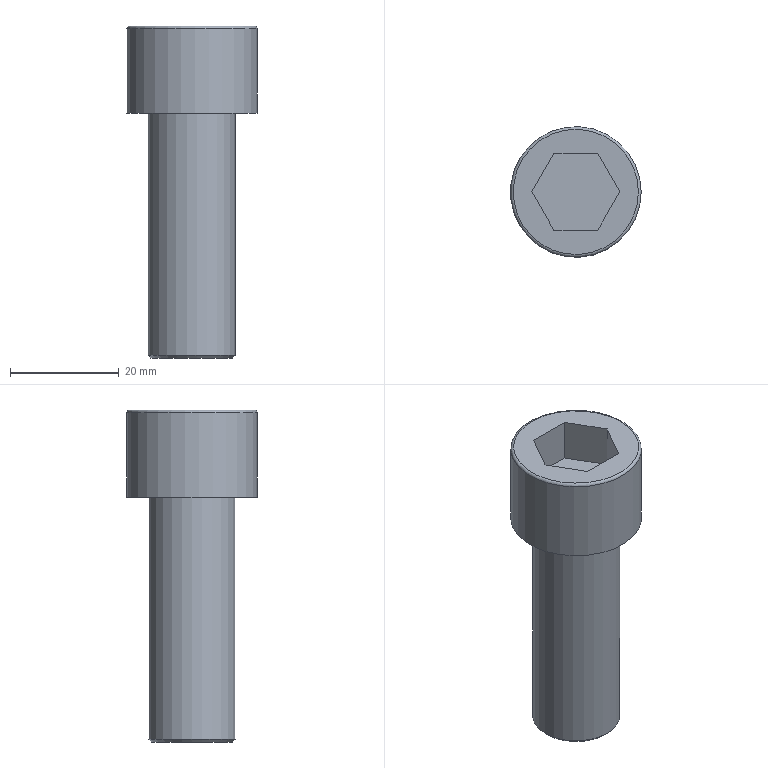Part | NX | features solid 2 | 1 solid | 14 faces | box 24 x 24 x 61 mm | volume 14918 mm3 | plane 10 | cylinder 2 | torus 1 | cone 1 | commonest cylinder face diameters 16 x1 24 x1
STEP:
#1=CARTESIAN_POINT('',(169.041,-134.,174.5));
#2=VERTEX_POINT('',#1);
#3=CARTESIAN_POINT('',(173.083,-127.,174.5));
#4=VERTEX_POINT('',#3);
#5=CARTESIAN_POINT('',(169.041,-134.,174.5));
#6=DIRECTION('',(0.5,0.866,0.));
#7=VECTOR('',#6,1000.);
#8=LINE('',#5,#7);
#9=EDGE_CURVE('',#2,#4,#8,.T.);
#10=ORIENTED_EDGE('',*,*,#9,.F.);
#11=CARTESIAN_POINT('',(160.959,-134.,174.5));
#12=VERTEX_POINT('',#11);
#13=CARTESIAN_POINT('',(160.959,-134.,174.5));
#14=DIRECTION('',(1.,0.,0.));
#15=VECTOR('',#14,1000.);
#16=LINE('',#13,#15);
#17=EDGE_CURVE('',#12,#2,#16,.T.);
#18=ORIENTED_EDGE('',*,*,#17,.F.);
#19=CARTESIAN_POINT('',(156.917,-127.,174.5));
#20=VERTEX_POINT('',#19);
#21=CARTESIAN_POINT('',(156.917,-127.,174.5));
#22=DIRECTION('',(0.5,-0.866,0.));
#23=VECTOR('',#22,1000.);
#24=LINE('',#21,#23);
#25=EDGE_CURVE('',#20,#12,#24,.T.);
#26=ORIENTED_EDGE('',*,*,#25,.F.);
#27=CARTESIAN_POINT('',(160.959,-120.,174.5));
#28=VERTEX_POINT('',#27);
#29=CARTESIAN_POINT('',(160.959,-120.,174.5));
#30=DIRECTION('',(-0.5,-0.866,0.));
#31=VECTOR('',#30,1000.);
#32=LINE('',#29,#31);
#33=EDGE_CURVE('',#28,#20,#32,.T.);
#34=ORIENTED_EDGE('',*,*,#33,.F.);
#35=CARTESIAN_POINT('',(169.041,-120.,174.5));
#36=VERTEX_POINT('',#35);
#37=CARTESIAN_POINT('',(169.041,-120.,174.5));
#38=DIRECTION('',(-1.,0.,0.));
#39=VECTOR('',#38,1000.);
#40=LINE('',#37,#39);
#41=EDGE_CURVE('',#36,#28,#40,.T.);
#42=ORIENTED_EDGE('',*,*,#41,.F.);
#43=CARTESIAN_POINT('',(173.083,-127.,174.5));
#44=DIRECTION('',(-0.5,0.866,0.));
#45=VECTOR('',#44,1000.);
#46=LINE('',#43,#45);
#47=EDGE_CURVE('',#4,#36,#46,.T.);
#48=ORIENTED_EDGE('',*,*,#47,.F.);
#49=EDGE_LOOP('',(#10,#18,#26,#34,#42,#48));
#50=FACE_BOUND('',#49,.T.);
#51=CARTESIAN_POINT('',(176.5,-127.,174.5));
#52=VERTEX_POINT('',#51);
#53=CARTESIAN_POINT('',(165.,-127.,174.5));
#54=DIRECTION('',(0.,0.,1.));
#55=DIRECTION('',(1.,0.,0.));
#56=AXIS2_PLACEMENT_3D('',#53,#54,#55);
#57=CIRCLE('',#56,11.5);
#58=EDGE_CURVE('',#52,#52,#57,.T.);
#59=ORIENTED_EDGE('',*,*,#58,.T.);
#60=EDGE_LOOP('',(#59));
#61=FACE_BOUND('',#60,.T.);
#62=CARTESIAN_POINT('',(165.,-127.,174.5));
#63=DIRECTION('',(0.,0.,1.));
#64=DIRECTION('',(1.,0.,0.));
#65=AXIS2_PLACEMENT_3D('',#62,#63,#64);
#66=PLANE('',#65);
#67=ADVANCED_FACE('',(#50,#61),#66,.T.);
#68=CARTESIAN_POINT('',(157.,-127.,158.5));
#69=VERTEX_POINT('',#68);
#70=CARTESIAN_POINT('',(165.,-127.,158.5));
#71=DIRECTION('',(0.,0.,-1.));
#72=DIRECTION('',(-1.,0.,0.));
#73=AXIS2_PLACEMENT_3D('',#70,#71,#72);
#74=CIRCLE('',#73,8.);
#75=EDGE_CURVE('',#69,#69,#74,.T.);
#76=ORIENTED_EDGE('',*,*,#75,.F.);
#77=EDGE_LOOP('',(#76));
#78=FACE_BOUND('',#77,.T.);
#79=CARTESIAN_POINT('',(177.,-127.,158.5));
#80=VERTEX_POINT('',#79);
#81=CARTESIAN_POINT('',(165.,-127.,158.5));
#82=DIRECTION('',(0.,0.,1.));
#83=DIRECTION('',(1.,0.,0.));
#84=AXIS2_PLACEMENT_3D('',#81,#82,#83);
#85=CIRCLE('',#84,12.);
#86=EDGE_CURVE('',#80,#80,#85,.T.);
#87=ORIENTED_EDGE('',*,*,#86,.F.);
#88=EDGE_LOOP('',(#87));
#89=FACE_BOUND('',#88,.T.);
#90=CARTESIAN_POINT('',(165.,-127.,158.5));
#91=DIRECTION('',(0.,0.,-1.));
#92=DIRECTION('',(-1.,0.,0.));
#93=AXIS2_PLACEMENT_3D('',#90,#91,#92);
#94=PLANE('',#93);
#95=ADVANCED_FACE('',(#78,#89),#94,.T.);
#96=CARTESIAN_POINT('',(177.,-127.,174.));
#97=VERTEX_POINT('',#96);
#98=CARTESIAN_POINT('',(165.,-127.,174.));
#99=DIRECTION('',(0.,0.,1.));
#100=DIRECTION('',(1.,0.,0.));
#101=AXIS2_PLACEMENT_3D('',#98,#99,#100);
#102=CIRCLE('',#101,12.);
#103=EDGE_CURVE('',#97,#97,#102,.F.);
#104=ORIENTED_EDGE('',*,*,#103,.T.);
#105=EDGE_LOOP('',(#104));
#106=FACE_BOUND('',#105,.T.);
#107=ORIENTED_EDGE('',*,*,#86,.T.);
#108=EDGE_LOOP('',(#107));
#109=FACE_BOUND('',#108,.T.);
#110=CARTESIAN_POINT('',(165.,-127.,158.5));
#111=DIRECTION('',(0.,0.,1.));
#112=DIRECTION('',(1.,0.,0.));
#113=AXIS2_PLACEMENT_3D('',#110,#111,#112);
#114=CYLINDRICAL_SURFACE('',#113,12.);
#115=ADVANCED_FACE('',(#106,#109),#114,.T.);
#116=ORIENTED_EDGE('',*,*,#58,.F.);
#117=EDGE_LOOP('',(#116));
#118=FACE_BOUND('',#117,.T.);
#119=ORIENTED_EDGE('',*,*,#103,.F.);
#120=EDGE_LOOP('',(#119));
#121=FACE_BOUND('',#120,.T.);
#122=CARTESIAN_POINT('',(165.,-127.,174.));
#123=DIRECTION('',(0.,0.,1.));
#124=DIRECTION('',(1.,0.,0.));
#125=AXIS2_PLACEMENT_3D('',#122,#123,#124);
#126=TOROIDAL_SURFACE('',#125,11.5,0.5);
#127=ADVANCED_FACE('',(#118,#121),#126,.T.);
#128=CARTESIAN_POINT('',(157.5,-127.,113.5));
#129=VERTEX_POINT('',#128);
#130=CARTESIAN_POINT('',(165.,-127.,113.5));
#131=DIRECTION('',(0.,0.,-1.));
#132=DIRECTION('',(-1.,0.,0.));
#133=AXIS2_PLACEMENT_3D('',#130,#131,#132);
#134=CIRCLE('',#133,7.5);
#135=EDGE_CURVE('',#129,#129,#134,.T.);
#136=ORIENTED_EDGE('',*,*,#135,.T.);
#137=EDGE_LOOP('',(#136));
#138=FACE_BOUND('',#137,.T.);
#139=CARTESIAN_POINT('',(165.,-127.,113.5));
#140=DIRECTION('',(0.,0.,-1.));
#141=DIRECTION('',(-1.,0.,0.));
#142=AXIS2_PLACEMENT_3D('',#139,#140,#141);
#143=PLANE('',#142);
#144=ADVANCED_FACE('',(#138),#143,.T.);
#145=CARTESIAN_POINT('',(157.,-127.,114.));
#146=VERTEX_POINT('',#145);
#147=CARTESIAN_POINT('',(165.,-127.,114.));
#148=DIRECTION('',(0.,0.,-1.));
#149=DIRECTION('',(-1.,0.,0.));
#150=AXIS2_PLACEMENT_3D('',#147,#148,#149);
#151=CIRCLE('',#150,8.);
#152=EDGE_CURVE('',#146,#146,#151,.F.);
#153=ORIENTED_EDGE('',*,*,#152,.T.);
#154=EDGE_LOOP('',(#153));
#155=FACE_BOUND('',#154,.T.);
#156=ORIENTED_EDGE('',*,*,#75,.T.);
#157=EDGE_LOOP('',(#156));
#158=FACE_BOUND('',#157,.T.);
#159=CARTESIAN_POINT('',(165.,-127.,113.5));
#160=DIRECTION('',(0.,0.,1.));
#161=DIRECTION('',(1.,0.,0.));
#162=AXIS2_PLACEMENT_3D('',#159,#160,#161);
#163=CYLINDRICAL_SURFACE('',#162,8.);
#164=ADVANCED_FACE('',(#155,#158),#163,.T.);
#165=ORIENTED_EDGE('',*,*,#135,.F.);
#166=EDGE_LOOP('',(#165));
#167=FACE_BOUND('',#166,.T.);
#168=ORIENTED_EDGE('',*,*,#152,.F.);
#169=EDGE_LOOP('',(#168));
#170=FACE_BOUND('',#169,.T.);
#171=CARTESIAN_POINT('',(165.,-127.,114.));
#172=DIRECTION('',(0.,0.,1.));
#173=DIRECTION('',(1.,0.,0.));
#174=AXIS2_PLACEMENT_3D('',#171,#172,#173);
#175=CONICAL_SURFACE('',#174,8.,0.7854);
#176=ADVANCED_FACE('',(#167,#170),#175,.T.);
#177=ORIENTED_EDGE('',*,*,#9,.T.);
#178=CARTESIAN_POINT('',(173.083,-127.,166.5));
#179=VERTEX_POINT('',#178);
#180=CARTESIAN_POINT('',(173.083,-127.,166.5));
#181=DIRECTION('',(0.,0.,1.));
#182=VECTOR('',#181,1000.);
#183=LINE('',#180,#182);
#184=EDGE_CURVE('',#179,#4,#183,.T.);
#185=ORIENTED_EDGE('',*,*,#184,.F.);
#186=CARTESIAN_POINT('',(169.041,-134.,166.5));
#187=VERTEX_POINT('',#186);
#188=CARTESIAN_POINT('',(169.041,-134.,166.5));
#189=DIRECTION('',(0.5,0.866,0.));
#190=VECTOR('',#189,1000.);
#191=LINE('',#188,#190);
#192=EDGE_CURVE('',#187,#179,#191,.T.);
#193=ORIENTED_EDGE('',*,*,#192,.F.);
#194=CARTESIAN_POINT('',(169.041,-134.,166.5));
#195=DIRECTION('',(0.,0.,1.));
#196=VECTOR('',#195,1000.);
#197=LINE('',#194,#196);
#198=EDGE_CURVE('',#187,#2,#197,.T.);
#199=ORIENTED_EDGE('',*,*,#198,.T.);
#200=EDGE_LOOP('',(#177,#185,#193,#199));
#201=FACE_BOUND('',#200,.T.);
#202=CARTESIAN_POINT('',(171.062,-130.5,170.5));
#203=DIRECTION('',(0.866,-0.5,0.));
#204=DIRECTION('',(0.5,0.866,0.));
#205=AXIS2_PLACEMENT_3D('',#202,#203,#204);
#206=PLANE('',#205);
#207=ADVANCED_FACE('',(#201),#206,.F.);
#208=ORIENTED_EDGE('',*,*,#17,.T.);
#209=ORIENTED_EDGE('',*,*,#198,.F.);
#210=CARTESIAN_POINT('',(160.959,-134.,166.5));
#211=VERTEX_POINT('',#210);
#212=CARTESIAN_POINT('',(160.959,-134.,166.5));
#213=DIRECTION('',(1.,0.,0.));
#214=VECTOR('',#213,1000.);
#215=LINE('',#212,#214);
#216=EDGE_CURVE('',#211,#187,#215,.T.);
#217=ORIENTED_EDGE('',*,*,#216,.F.);
#218=CARTESIAN_POINT('',(160.959,-134.,166.5));
#219=DIRECTION('',(0.,0.,1.));
#220=VECTOR('',#219,1000.);
#221=LINE('',#218,#220);
#222=EDGE_CURVE('',#211,#12,#221,.T.);
#223=ORIENTED_EDGE('',*,*,#222,.T.);
#224=EDGE_LOOP('',(#208,#209,#217,#223));
#225=FACE_BOUND('',#224,.T.);
#226=CARTESIAN_POINT('',(165.,-134.,170.5));
#227=DIRECTION('',(0.,-1.,0.));
#228=DIRECTION('',(0.,0.,-1.));
#229=AXIS2_PLACEMENT_3D('',#226,#227,#228);
#230=PLANE('',#229);
#231=ADVANCED_FACE('',(#225),#230,.F.);
#232=ORIENTED_EDGE('',*,*,#25,.T.);
#233=ORIENTED_EDGE('',*,*,#222,.F.);
#234=CARTESIAN_POINT('',(156.917,-127.,166.5));
#235=VERTEX_POINT('',#234);
#236=CARTESIAN_POINT('',(156.917,-127.,166.5));
#237=DIRECTION('',(0.5,-0.866,0.));
#238=VECTOR('',#237,1000.);
#239=LINE('',#236,#238);
#240=EDGE_CURVE('',#235,#211,#239,.T.);
#241=ORIENTED_EDGE('',*,*,#240,.F.);
#242=CARTESIAN_POINT('',(156.917,-127.,166.5));
#243=DIRECTION('',(0.,0.,1.));
#244=VECTOR('',#243,1000.);
#245=LINE('',#242,#244);
#246=EDGE_CURVE('',#235,#20,#245,.T.);
#247=ORIENTED_EDGE('',*,*,#246,.T.);
#248=EDGE_LOOP('',(#232,#233,#241,#247));
#249=FACE_BOUND('',#248,.T.);
#250=CARTESIAN_POINT('',(158.938,-130.5,170.5));
#251=DIRECTION('',(-0.866,-0.5,0.));
#252=DIRECTION('',(0.5,-0.866,0.));
#253=AXIS2_PLACEMENT_3D('',#250,#251,#252);
#254=PLANE('',#253);
#255=ADVANCED_FACE('',(#249),#254,.F.);
#256=ORIENTED_EDGE('',*,*,#33,.T.);
#257=ORIENTED_EDGE('',*,*,#246,.F.);
#258=CARTESIAN_POINT('',(160.959,-120.,166.5));
#259=VERTEX_POINT('',#258);
#260=CARTESIAN_POINT('',(160.959,-120.,166.5));
#261=DIRECTION('',(-0.5,-0.866,0.));
#262=VECTOR('',#261,1000.);
#263=LINE('',#260,#262);
#264=EDGE_CURVE('',#259,#235,#263,.T.);
#265=ORIENTED_EDGE('',*,*,#264,.F.);
#266=CARTESIAN_POINT('',(160.959,-120.,166.5));
#267=DIRECTION('',(0.,0.,1.));
#268=VECTOR('',#267,1000.);
#269=LINE('',#266,#268);
#270=EDGE_CURVE('',#259,#28,#269,.T.);
#271=ORIENTED_EDGE('',*,*,#270,.T.);
#272=EDGE_LOOP('',(#256,#257,#265,#271));
#273=FACE_BOUND('',#272,.T.);
#274=CARTESIAN_POINT('',(158.938,-123.5,170.5));
#275=DIRECTION('',(-0.866,0.5,0.));
#276=DIRECTION('',(-0.5,-0.866,0.));
#277=AXIS2_PLACEMENT_3D('',#274,#275,#276);
#278=PLANE('',#277);
#279=ADVANCED_FACE('',(#273),#278,.F.);
#280=ORIENTED_EDGE('',*,*,#41,.T.);
#281=ORIENTED_EDGE('',*,*,#270,.F.);
#282=CARTESIAN_POINT('',(169.041,-120.,166.5));
#283=VERTEX_POINT('',#282);
#284=CARTESIAN_POINT('',(169.041,-120.,166.5));
#285=DIRECTION('',(-1.,0.,0.));
#286=VECTOR('',#285,1000.);
#287=LINE('',#284,#286);
#288=EDGE_CURVE('',#283,#259,#287,.T.);
#289=ORIENTED_EDGE('',*,*,#288,.F.);
#290=CARTESIAN_POINT('',(169.041,-120.,166.5));
#291=DIRECTION('',(0.,0.,1.));
#292=VECTOR('',#291,1000.);
#293=LINE('',#290,#292);
#294=EDGE_CURVE('',#283,#36,#293,.T.);
#295=ORIENTED_EDGE('',*,*,#294,.T.);
#296=EDGE_LOOP('',(#280,#281,#289,#295));
#297=FACE_BOUND('',#296,.T.);
#298=CARTESIAN_POINT('',(165.,-120.,170.5));
#299=DIRECTION('',(0.,1.,0.));
#300=DIRECTION('',(0.,0.,1.));
#301=AXIS2_PLACEMENT_3D('',#298,#299,#300);
#302=PLANE('',#301);
#303=ADVANCED_FACE('',(#297),#302,.F.);
#304=ORIENTED_EDGE('',*,*,#47,.T.);
#305=ORIENTED_EDGE('',*,*,#294,.F.);
#306=CARTESIAN_POINT('',(173.083,-127.,166.5));
#307=DIRECTION('',(-0.5,0.866,0.));
#308=VECTOR('',#307,1000.);
#309=LINE('',#306,#308);
#310=EDGE_CURVE('',#179,#283,#309,.T.);
#311=ORIENTED_EDGE('',*,*,#310,.F.);
#312=ORIENTED_EDGE('',*,*,#184,.T.);
#313=EDGE_LOOP('',(#304,#305,#311,#312));
#314=FACE_BOUND('',#313,.T.);
#315=CARTESIAN_POINT('',(171.062,-123.5,170.5));
#316=DIRECTION('',(0.866,0.5,0.));
#317=DIRECTION('',(-0.5,0.866,0.));
#318=AXIS2_PLACEMENT_3D('',#315,#316,#317);
#319=PLANE('',#318);
#320=ADVANCED_FACE('',(#314),#319,.F.);
#321=ORIENTED_EDGE('',*,*,#310,.T.);
#322=ORIENTED_EDGE('',*,*,#288,.T.);
#323=ORIENTED_EDGE('',*,*,#264,.T.);
#324=ORIENTED_EDGE('',*,*,#240,.T.);
#325=ORIENTED_EDGE('',*,*,#216,.T.);
#326=ORIENTED_EDGE('',*,*,#192,.T.);
#327=EDGE_LOOP('',(#321,#322,#323,#324,#325,#326));
#328=FACE_BOUND('',#327,.T.);
#329=CARTESIAN_POINT('',(165.,-127.,166.5));
#330=DIRECTION('',(0.,0.,-1.));
#331=DIRECTION('',(-1.,0.,0.));
#332=AXIS2_PLACEMENT_3D('',#329,#330,#331);
#333=PLANE('',#332);
#334=ADVANCED_FACE('',(#328),#333,.F.);
#335=CLOSED_SHELL('',(#67,#95,#115,#127,#144,#164,#176,#207,#231,#255,#279,#303,#320,#334));
#336=MANIFOLD_SOLID_BREP('',#335);
#337=(LENGTH_UNIT()NAMED_UNIT(*)SI_UNIT(.MILLI.,.METRE.));
#338=UNCERTAINTY_MEASURE_WITH_UNIT(LENGTH_MEASURE(0.00001),#337,'','');
#339=(NAMED_UNIT(*)PLANE_ANGLE_UNIT()SI_UNIT($,.RADIAN.));
#340=(NAMED_UNIT(*)SI_UNIT($,.STERADIAN.)SOLID_ANGLE_UNIT());
#341=(GEOMETRIC_REPRESENTATION_CONTEXT(3)GLOBAL_UNCERTAINTY_ASSIGNED_CONTEXT((#338))GLOBAL_UNIT_ASSIGNED_CONTEXT((#337,#339,#340))REPRESENTATION_CONTEXT('',''));
#342=ADVANCED_BREP_SHAPE_REPRESENTATION('',(#336),#341);